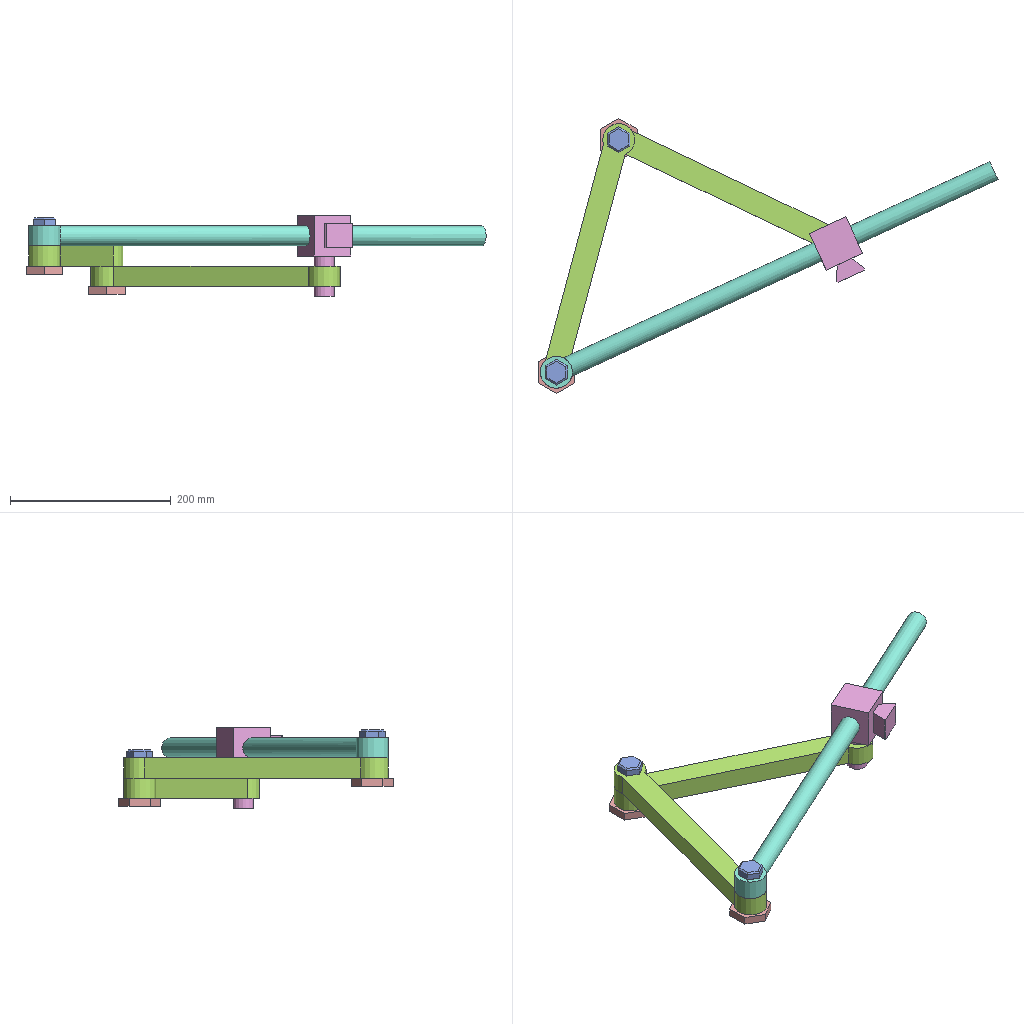Assembly | NX | 6 different items | 9 placed | box 573 x 343 x 100 mm
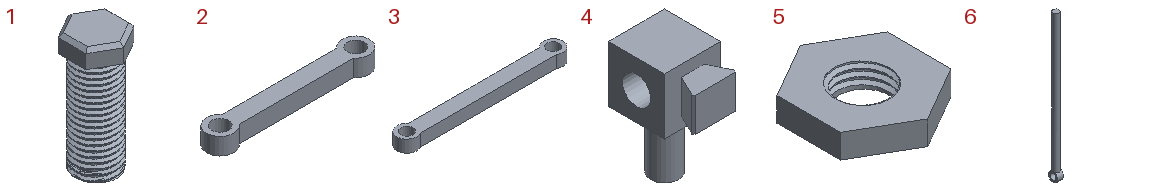Parts list (item | quantity | size | volume | features):
1 | x2 | 27.713 x 32 x 70 mm | 30636 mm3 | features DATUM_CSYS 3, EXTRUDE 2, SKETCH 2, CHAMFER 1, THREADS 1
2 | x1 | 240 x 40 x 25 mm | 140028 mm3 | features DATUM_CSYS 2, SIMPLE HOLE 2, EXTRUDE 1, HOLE PACKAGE 1, SKETCH 1
3 | x2 | - | 232729 mm3 | features DATUM_CSYS 2, SIMPLE HOLE 2, EXTRUDE 1, HOLE PACKAGE 1, SKETCH 1
4 | x1 | 50 x 70 x 100 mm | 142893 mm3 | features DATUM_CSYS 4, EXTRUDE 4, SKETCH 3, CHAMFER 1
5 | x2 | 45.899 x 53 x 10 mm | 14258 mm3 | features DATUM_CSYS 2, EXTRUDE 1, SKETCH 1, THREADS 1
6 | x1 | 25 x 40 x 620 mm | 304356 mm3 | features DATUM_CSYS 3, EXTRUDE 2, SKETCH 2, HOLE PACKAGE 1, SIMPLE HOLE 1
Mates (type | each side: item.copy, entity, surface, feature):
Touch | 6.1 face cylinder Extrude(2) | 4.1 face cylinder Extrude(6)
Parallel | 6.1 face plane Extrude(4) | 4.1 face plane Extrude(2)
Concentric | 3.1 edge | 6.1 edge
Concentric | 3.1 edge | 3.1 edge
Touch | 3.1 face cylinder Ø25 Hole(4) | 4.1 face cylinder Extrude(8)
Touch | 1.1 face cylinder Extrude(3) | 6.1 face cylinder Extrude(4)
Touch | 1.1 face plane Extrude(4) | 6.1 face plane Extrude(4)
Touch | 5.1 face cylinder Extrude(2) | 1.1 face cylinder Extrude(3)
Touch | 5.1 face plane Extrude(2) | 3.1 face plane Extrude(3)